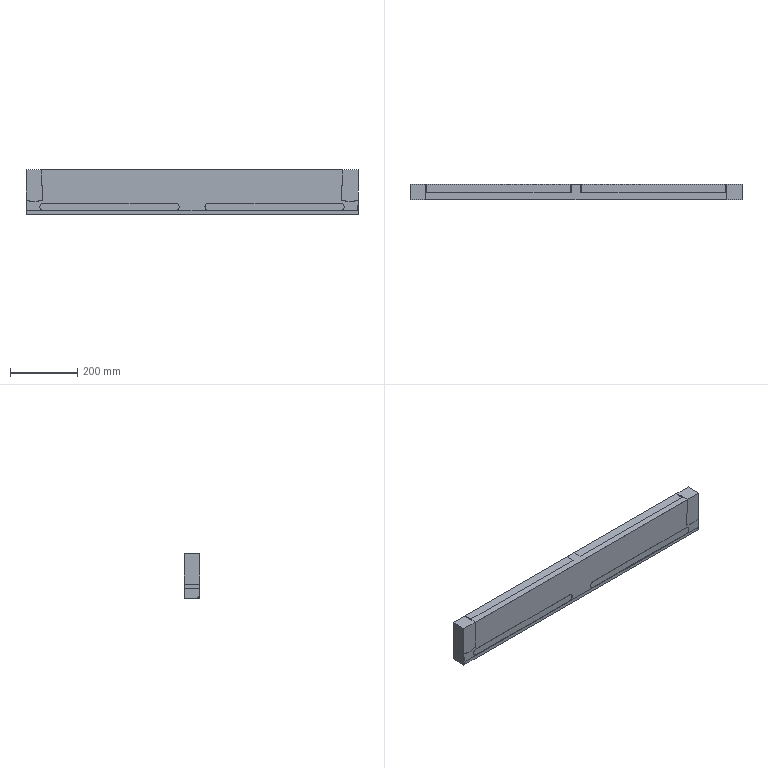Part | 2 solids | 113 faces | box 987 x 45 x 132.5 mm | volume 10530822 mm3 | plane 56 | cylinder 31 | cone 26 | commonest cylinder face diameters 6.8 x16 21 x6 20 x5 8 x4